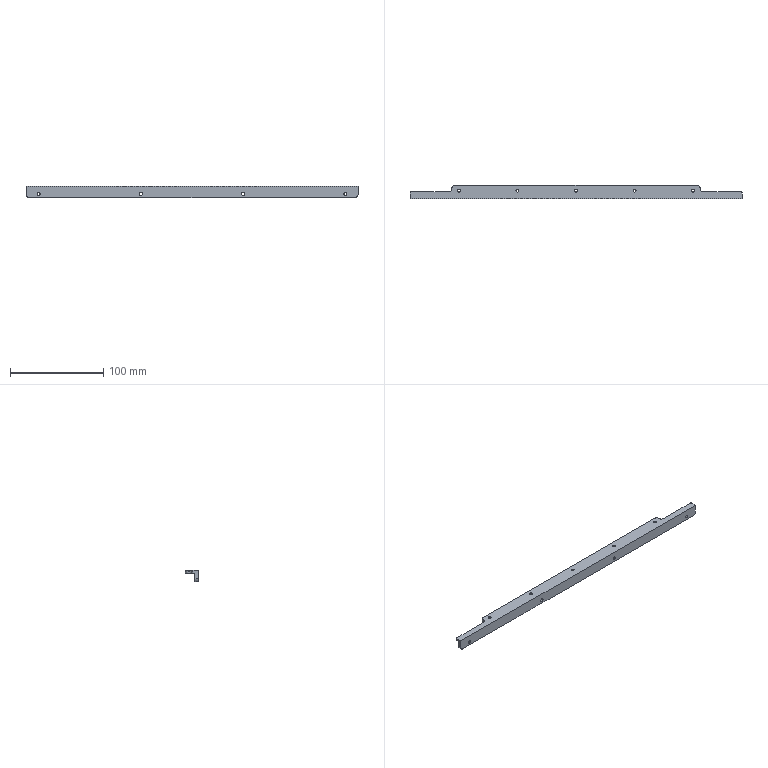NC program | NX | posted with a generic post | part box 356.96 x 14 x 12 mm
Lines 2604 to 3585 of 3585:
(PLANAR_MILL_1 , TOOL : D6精光)
N5200 T02 M6
N5202 G54
N5204 G17 G0 G90 X-181.515 Y-11.197 B0. C0. S4500 M3
N5206 G43 Z30. H2
N5208 Z-10.2
N5210 G94 G1 Z-12.2 F800.
N5212 G41 X-181.48 Y-11.
N5214 Y-6.998
N5216 Y-1.
N5218 G2 X-177.48 Y3. R4.
N5220 G1 X-136.5
N5222 Y4.
N5224 G2 X-130.5 Y10. R6.
N5226 G1 X130.5
N5228 G2 X136.5 Y4. R6.
N5230 G1 Y3.
N5232 X177.48
N5234 G2 X181.48 Y-1. R4.
N5236 G1 Y-7.
N5238 G2 X178.48 Y-10. R3.
N5240 G1 X-178.478
N5242 X-182.48
N5244 G40
N5246 X-182.677 Y-10.035
N5248 Z-10.2
N5250 G0 Z30.
N5252 X-181.515 Y-11.197
N5254 Z-10.2
N5256 G1 Z-12.2
N5258 G41 X-181.48 Y-11.
N5260 Y-6.998
N5262 Y-1.
N5264 G2 X-177.48 Y3. R4.
N5266 G1 X-136.5
N5268 Y4.
N5270 G2 X-130.5 Y10. R6.
N5272 G1 X130.5
N5274 G2 X136.5 Y4. R6.
N5276 G1 Y3.
N5278 X177.48
N5280 G2 X181.48 Y-1. R4.
N5282 G1 Y-7.
N5284 G2 X178.48 Y-10. R3.
N5286 G1 X-178.478
N5288 X-182.48
N5290 G40
N5292 X-182.677 Y-10.035
N5294 Z-10.2
N5296 G0 Z30.
(FLOOR_FACING , TOOL : D6精光)
N5298 X-137.886 Y9.315
N5300 Z-6.
N5302 G1 Z-9.
N5304 Y7.1
N5306 G3 X-136.386 Y5.6 R1.5
N5308 G1 X136.386
N5310 X177.48 Y3.1
N5312 X178.196 Y3.037
N5314 X178.89 Y2.85
N5316 X-178.89
N5318 G3 X-181.43 Y0.1 R4.1
N5320 G1 X181.43
N5322 G3 X182.93 Y1.6 R1.5
N5324 G1 Y3.551
N5326 Z-6.
N5328 G0 Z30.
(PLANAR_MILL_1_COPY , TOOL : D6精光)
N5330 X-183.677 Y0.035
N5332 Z-7.
N5334 G1 Z-9.
N5336 G41 X-183.48 Y0.
N5338 X-178.48
N5340 X178.48
N5342 X183.48
N5344 G40
N5346 X183.677 Y0.035
N5348 Z-7.
N5350 G0 Z30.
N5352 M5
(DRILLING , TOOL : D6点钻)
N5354 T03 M6
N5356 G54
N5358 G17 G0 G90 X-126. Y1.5 B0. C0. S3000 M3
N5360 G43 Z30. H3
N5362 G94 G81 G98 Z-11.5 F200. R-6.
N5364 X-63.
N5366 X0.
N5368 X63.
N5370 X126.
N5372 G80
N5374 G0 X126. Y1.5 Z30.
(PLANAR_MILL_2 , TOOL : D6点钻)
N5376 X-178.98 Y-1.5 S3500
N5378 Z0.5
N5380 G1 Z-1.5 F1000.
N5382 X-175.48
N5384 X175.48
N5386 X178.98
N5388 Z0.5
N5390 G0 Z30.
N5392 Y-8.5
N5394 Z0.5
N5396 G1 Z-1.5
N5398 X175.48
N5400 X-175.48
N5402 X-178.98
N5404 Z0.5
N5406 G0 Z30.
(PLANAR_MILL_2_COPY , TOOL : D6点钻)
N5408 X-181.48 Y2.
N5410 Z-9.
N5412 G1 Z-11.
N5414 X-177.48
N5416 X-136.5
N5418 G3 X-135.5 Y3. R1.
N5420 G1 Y4.
N5422 G2 X-130.5 Y9. R5.
N5424 G1 X130.5
N5426 G2 X135.5 Y4. R5.
N5428 G1 Y3.
N5430 G3 X136.5 Y2. R1.
N5432 G1 X177.48
N5434 X181.48
N5436 Z-9.
N5438 G0 Z30.
N5440 M5
(DRILLING_COPY , TOOL : D3.2)
N5442 T04 M6
N5444 G54
N5446 G17 G0 G90 X-126. Y1.5 B0. C0. S3000 M3
N5448 G43 Z30. H4
N5450 G94 G81 G98 Z-15. F200. R-6.
N5452 X-63.
N5454 X0.
N5456 X63.
N5458 X126.
N5460 G80
N5462 G0 X126. Y1.5 Z30.
N5464 M5
(CURVE_DRIVE , TOOL : D4R0.5)
N5466 T05 M6
N5468 G54
N5470 G17 G0 G90 X-180.431 Y-8.996 B0. C0. S4500 M3
N5472 G43 Z30. H5
N5474 Z1.526
N5476 G94 G1 Z-1.437 F1500.
N5478 X-180.433 Y-8.899 Z-2.055
N5480 X-180.439 Y-8.616 Z-2.613
N5482 X-180.448 Y-8.174 Z-3.056
N5484 X-180.46 Y-7.617 Z-3.341
N5486 X-180.473 Y-7. Z-3.44
N5488 X-180.476 Y-3.147 Z-3.441
N5490 X-180.468 Y-3.059 Z-3.44
N5492 X-180.465 Y-2.995 Z-3.474
N5494 X-180.468 Y-3.059 Z-3.44
N5496 X-180.47 Y-3.078
N5498 Y-3.106 Z-3.394
N5500 Y-3.123 Z-3.384
N5502 Y-6.878
N5504 Y-7. Z-3.408
N5506 X-180.463 Z-3.35
N5508 Y-6.845 Z-3.326
N5510 Y-3.155
N5512 Y-3.097 Z-3.331
N5514 Y-3.067 Z-3.348
N5516 Y-3.038 Z-3.387
N5518 Y-3.024 Z-3.419
N5520 Y-2.995 Z-3.456
N5522 X-180.457 Y-2.996 Z-3.346
N5524 Y-3.028 Z-3.303
N5526 Y-3.07 Z-3.279
N5528 Y-3.155 Z-3.271
N5530 Y-6.845
N5532 Y-7. Z-3.292
N5534 X-180.451 Z-3.234
N5536 Y-6.845 Z-3.215
N5538 Y-3.155
N5540 Y-3.044 Z-3.225
N5542 Y-2.997 Z-3.252
N5544 X-180.444 Y-2.998 Z-3.183
N5546 Y-3.018 Z-3.172
N5548 Y-3.155 Z-3.159
N5550 Y-6.845
N5552 Y-7. Z-3.175
N5554 X-180.437 Z-3.115
N5556 Y-6.845 Z-3.1
N5558 Y-3.155
N5560 Y-2.999 Z-3.115
N5562 X-180.43 Y-3. Z-3.055
N5564 Y-3.155 Z-3.04
N5566 Y-6.845
N5568 Y-7. Z-3.055
N5570 X-180.424 Z-2.996
N5572 Y-6.845 Z-2.981
N5574 Y-3.155
N5576 Y-3. Z-2.996
N5578 X-180.417 Z-2.936
N5580 Y-3.155 Z-2.921
N5582 Y-6.845
N5584 Y-7. Z-2.936
N5586 X-180.41 Z-2.876
N5588 Y-6.845 Z-2.862
N5590 Y-3.155
N5592 Y-3. Z-2.876
N5594 X-180.403 Y-3.001 Z-2.817
N5596 Y-3.154 Z-2.802
N5598 Y-6.842
N5600 Y-7. Z-2.817
N5602 X-180.385 Z-2.759
N5604 Y-6.845 Z-2.745
N5606 Y-3.155
N5608 Y-3.001 Z-2.759
N5610 X-180.367 Z-2.702
N5612 Y-3.155 Z-2.687
N5614 Y-6.845
N5616 Y-6.999 Z-2.702
N5618 X-180.349 Z-2.645
N5620 Y-6.845 Z-2.63
N5622 Y-3.155
N5624 Y-3.001 Z-2.645
N5626 X-180.331 Z-2.588
N5628 Y-3.155 Z-2.573
N5630 Y-6.845
N5632 Y-6.999 Z-2.588
N5634 X-180.313 Z-2.534
N5636 Y-6.845 Z-2.516
N5638 Y-3.155
N5640 Y-3.002 Z-2.534
N5642 X-180.295 Z-2.481
N5644 Y-3.067 Z-2.467
N5646 Y-3.155 Z-2.458
N5648 Y-6.845
N5650 Y-6.933 Z-2.467
N5652 Y-6.999 Z-2.481
N5654 X-180.277 Z-2.428
N5656 Y-6.897 Z-2.406
N5658 Y-6.845 Z-2.401
N5660 Y-3.155
N5662 Y-3.104 Z-2.406
N5664 Y-3.002 Z-2.428
N5666 X-180.259 Y-3.001 Z-2.375
N5668 Y-3.155 Z-2.344
N5670 Y-6.86 Z-2.345
N5672 Y-6.999 Z-2.375
N5674 X-180.238 Z-2.321
N5676 Y-6.845 Z-2.288
N5678 Y-3.155
N5680 Y-3.001 Z-2.321
N5682 X-180.216 Z-2.265
N5684 Y-3.155 Z-2.232
N5686 Y-6.845
N5688 Y-6.999 Z-2.265
N5690 X-180.193 Z-2.21
N5692 Y-6.845 Z-2.177
N5694 Y-3.155
N5696 Y-3.001 Z-2.21
N5698 X-180.17 Z-2.155
N5700 Y-3.155 Z-2.121
N5702 Y-6.845
N5704 Y-6.999 Z-2.155
N5706 X-180.147 Z-2.099
N5708 Y-6.845 Z-2.066
N5710 Y-3.155
N5712 Y-3.001 Z-2.099
N5714 X-180.124 Z-2.044
N5716 Y-3.155 Z-2.011
N5718 Y-6.845
N5720 Y-6.999 Z-2.044
N5722 X-180.102 Z-1.99
N5724 X-180.101 Y-6.84 Z-1.955
N5726 Y-3.151 Z-1.956
N5728 Y-3.001 Z-1.988
N5730 X-180.076 Z-1.932
N5732 Y-3.155 Z-1.908
N5734 Y-6.845
N5736 Y-6.999 Z-1.932
N5738 X-180.051 Z-1.878
N5740 X-180.05 Y-6.845 Z-1.857
N5742 Y-3.155
N5744 Y-3.001 Z-1.877
N5746 X-180.023 Z-1.823
N5748 Y-3.155 Z-1.804
N5750 Y-6.845
N5752 Y-7. Z-1.823
N5754 X-179.995 Z-1.77
N5756 Y-6.845 Z-1.75
N5758 Y-3.155
N5760 Y-3. Z-1.77
N5762 X-179.968 Z-1.717
N5764 Y-3.155 Z-1.697
N5766 Y-6.845
N5768 Y-7.001 Z-1.717
N5770 X-179.938 Z-1.664
N5772 Y-6.845 Z-1.647
N5774 Y-3.128 Z-1.648
N5776 Y-3. Z-1.664
N5778 X-179.904 Z-1.614
N5780 Y-3.155 Z-1.604
N5782 Y-6.94 Z-1.606
N5784 Y-7.001 Z-1.614
N5786 X-179.871 Z-1.564
N5788 Y-5. Z-1.56
N5790 Y-3. Z-1.564
N5792 X-179.834 Z-1.516
N5794 Y-5. Z-1.512
N5796 Y-7. Z-1.516
N5798 X-179.798 Z-1.469
N5800 Y-4.997 Z-1.465
N5802 Y-3. Z-1.469
N5804 X-179.761 Z-1.421
N5806 Y-5. Z-1.417
N5808 Y-7.001 Z-1.421
N5810 X-179.725 Z-1.374
N5812 Y-5. Z-1.37
N5814 Y-2.999 Z-1.374
N5816 X-179.688 Z-1.326
N5818 Y-5. Z-1.322
N5820 Y-7.001 Z-1.326
N5822 X-179.653 Z-1.28
N5824 X-179.652 Y-6.845 Z-1.274
N5826 Y-3.155
N5828 Y-2.999 Z-1.279
N5830 X-179.615 Z-1.235
N5832 Y-3.155 Z-1.227
N5834 Y-6.963 Z-1.23
N5836 Y-7.001 Z-1.235
N5838 X-179.579 Y-7.002 Z-1.191
N5840 Y-6.845 Z-1.179
N5842 Y-3.075 Z-1.181
N5844 Y-2.999 Z-1.191
N5846 X-179.542 Y-2.998 Z-1.146
N5848 Y-3.155 Z-1.132
N5850 Y-6.888 Z-1.133
N5852 Y-7.002 Z-1.146
N5854 X-179.506 Z-1.102
N5856 Y-6.851 Z-1.084
N5858 Y-3.149
N5860 Y-2.998 Z-1.102
N5862 X-179.462 Z-1.06
N5864 Y-3.155 Z-1.045
N5866 Y-6.845
N5868 Y-7.002 Z-1.06
N5870 X-179.418 Y-7.001 Z-1.02
N5872 Y-6.845 Z-1.008
N5874 Y-3.155
N5876 Y-2.999 Z-1.02
N5878 X-179.372 Y-3. Z-0.981
N5880 Y-3.155 Z-0.969
N5882 Y-6.845
N5884 Y-7.001 Z-0.981
N5886 X-179.326 Y-7. Z-0.942
N5888 Y-6.845 Z-0.931
N5890 Y-3.155
N5892 Y-3. Z-0.942
N5894 X-179.281 Y-3.001 Z-0.903
N5896 Y-3.155 Z-0.892
N5898 Y-6.845
N5900 Y-6.999 Z-0.904
N5902 X-179.235 Y-7. Z-0.865
N5904 Y-6.845 Z-0.853
N5906 Y-3.155
N5908 Y-3.001 Z-0.865
N5910 X-179.188 Z-0.827
N5912 Y-3.155 Z-0.815
N5914 Y-6.845
N5916 Y-7. Z-0.827
N5918 X-179.141 Z-0.79
N5920 Y-6.845 Z-0.779
N5922 Y-3.155
N5924 Y-3.001 Z-0.79
N5926 X-179.093 Z-0.754
N5928 Y-3.155 Z-0.742
N5930 Y-6.845
N5932 Y-7. Z-0.754
N5934 X-179.046 Z-0.717
N5936 Y-6.845 Z-0.706
N5938 Y-3.155
N5940 Y-3.001 Z-0.717
N5942 X-178.998 Z-0.681
N5944 Y-3.155 Z-0.669
N5946 Y-6.845
N5948 Y-7. Z-0.681
N5950 X-178.95 Z-0.644
N5952 Y-6.845 Z-0.633
N5954 Y-3.155
N5956 Y-3.001 Z-0.644
N5958 X-178.903 Z-0.608
N5960 Y-3.153 Z-0.596
N5962 Y-6.845
N5964 Y-7. Z-0.608
N5966 X-178.853 Z-0.574
N5968 Y-6.845 Z-0.565
N5970 Y-3.155
N5972 Y-3.001 Z-0.574
N5974 X-178.803 Z-0.541
N5976 Y-3.155 Z-0.534
N5978 Y-6.845
N5980 Y-7. Z-0.541
N5982 X-178.751 Z-0.51
N5984 Y-6.845 Z-0.503
N5986 Y-3.155
N5988 Y-3.001 Z-0.51
N5990 X-178.7 Y-3. Z-0.479
N5992 Y-3.155 Z-0.472
N5994 Y-6.845
N5996 Y-7. Z-0.479
N5998 X-178.649 Z-0.448
N6000 Y-6.845 Z-0.441
N6002 Y-3.155
N6004 Y-3. Z-0.447
N6006 X-178.598 Z-0.416
N6008 Y-3.154 Z-0.41
N6010 Y-6.843
N6012 Y-7. Z-0.416
N6014 X-178.542 Z-0.393
N6016 Y-6.845 Z-0.387
N6018 Y-3.155
N6020 Y-3. Z-0.393
N6022 X-178.487 Z-0.37
N6024 Y-3.155 Z-0.364
N6026 Y-6.845
N6028 Y-7. Z-0.37
N6030 X-178.431 Z-0.347
N6032 Y-6.845 Z-0.341
N6034 Y-3.155
N6036 Y-3. Z-0.347
N6038 X-178.376 Z-0.324
N6040 Y-3.155 Z-0.318
N6042 Y-6.845
N6044 Y-7. Z-0.324
N6046 X-178.321 Z-0.301
N6048 Y-6.845 Z-0.295
N6050 Y-3.155
N6052 Y-3. Z-0.301
N6054 X-178.265 Z-0.278
N6056 Y-3.155 Z-0.272
N6058 Y-6.845
N6060 Y-7. Z-0.278
N6062 X-178.21 Z-0.255
N6064 Y-6.845 Z-0.249
N6066 Y-3.155
N6068 Y-3. Z-0.255
N6070 X-178.154 Z-0.232
N6072 Y-3.155 Z-0.226
N6074 Y-6.845
N6076 Y-7. Z-0.232
N6078 X-178.099 Z-0.21
N6080 Y-6.845 Z-0.203
N6082 Y-3.155
N6084 Y-3. Z-0.21
N6086 X-178.043 Z-0.187
N6088 Y-3.155 Z-0.18
N6090 Y-6.845
N6092 Y-7.001 Z-0.187
N6094 X-177.988 Z-0.164
N6096 Y-6.845 Z-0.158
N6098 Y-3.151
N6100 Y-3. Z-0.164
N6102 X-177.93 Z-0.147
N6104 Y-6.845 Z-0.143
N6106 Y-7.001 Z-0.147
N6108 X-177.873 Y-7. Z-0.131
N6110 Y-3.
N6112 X-177.815 Z-0.115
N6114 Y-7.
N6116 X-177.757 Z-0.1
N6118 Y-3.
N6120 X-177.699 Z-0.085
N6122 Y-7.
N6124 X-177.64 Z-0.073
N6126 Y-3.
N6128 X-177.581 Z-0.062
N6130 Y-7.
N6132 X-177.522 Z-0.051
N6134 Y-3.
N6136 X-177.463 Z-0.04
N6138 Y-7.
N6140 X-177.404 Z-0.03
N6142 Y-3.
N6144 X-177.344 Z-0.025
N6146 Y-7.
N6148 X-177.284 Z-0.022
N6150 Y-3.
N6152 X-177.224 Z-0.019
N6154 Y-7.
N6156 X-177.164 Z-0.016
N6158 Y-3.
N6160 X-177.104 Z-0.014
N6162 Y-7.
N6164 X-177.044 Z-0.011
N6166 Y-3.
N6168 X-176.984 Z-0.008
N6170 Y-7.
N6172 X-176.924 Z-0.006
N6174 Y-3.
N6176 X-176.864 Z-0.003
N6178 Y-7.
N6180 X-176.804 Z-0.001
N6182 Y-3.
N6184 X-176.744 Z0.
N6186 Y-7.
N6188 X-176.684
N6190 Y-3.
N6192 X-176.624
N6194 Y-7.
N6196 X-176.564
N6198 Y-3.
N6200 X-176.504
N6202 Y-7.
N6204 X-176.444
N6206 Y-3.
N6208 X-176.384
N6210 Y-7.
N6212 X-176.324
N6214 Y-3.
N6216 X-176.264
N6218 Y-7.
N6220 X-176.204
N6222 Y-3.
N6224 X-176.144
N6226 Y-7.
N6228 X-176.084
N6230 Y-3.
N6232 X-176.024
N6234 Y-7.
N6236 X-175.964
N6238 Y-3.
N6240 X-175.904
N6242 Y-7.
N6244 X-175.844
N6246 Y-3.
N6248 X-175.784
N6250 Y-7.
N6252 X-175.724
N6254 Y-3.
N6256 X-175.664
N6258 Y-7.
N6260 X-175.604
N6262 Y-3.
N6264 X-175.544
N6266 Y-7.
N6268 Y-7.618 Z0.098
N6270 Y-8.176 Z0.382
N6272 Y-8.618 Z0.824
N6274 Y-8.902 Z1.382
N6276 Y-9. Z2.
N6278 Z2.931
N6280 G0 Z30.
N6282 X175.57
N6284 Z2.93
N6286 G1 Z2.
N6288 Y-8.902 Z1.382
N6290 Y-8.618 Z0.824
N6292 Y-8.176 Z0.382
N6294 Y-7.618 Z0.098
N6296 Y-7. Z0.
N6298 Y-3.
N6300 X175.63
N6302 Y-7.
N6304 X175.69
N6306 Y-3.
N6308 X175.75
N6310 Y-7.
N6312 X175.81
N6314 Y-3.
N6316 X175.87
N6318 Y-7.
N6320 X175.93
N6322 Y-3.
N6324 X175.99
N6326 Y-7.
N6328 X176.05
N6330 Y-3.
N6332 X176.11
N6334 Y-7.
N6336 X176.17
N6338 Y-3.
N6340 X176.23
N6342 Y-7.
N6344 X176.29
N6346 Y-3.
N6348 X176.35
N6350 Y-7.
N6352 X176.41
N6354 Y-3.
N6356 X176.47
N6358 Y-7.
N6360 X176.53
N6362 Y-3.
N6364 X176.59
N6366 Y-7.
N6368 X176.65
N6370 Y-3.
N6372 X176.71
N6374 Y-7.
N6376 X176.77
N6378 Y-3.
N6380 X176.83 Z-0.002
N6382 Y-7.
N6384 X176.89 Z-0.004
N6386 Y-3.
N6388 X176.95 Z-0.007
N6390 Y-7.
N6392 X177.01 Z-0.009
N6394 Y-3.
N6396 X177.07 Z-0.012
N6398 Y-7.
N6400 X177.13 Z-0.015
N6402 Y-3.
N6404 X177.19 Z-0.017
N6406 Y-7.
N6408 X177.249 Z-0.02
N6410 Y-3.
N6412 X177.309 Z-0.023
N6414 Y-7.
N6416 X177.369 Z-0.027
N6418 Y-3.
N6420 X177.429 Z-0.034
N6422 Y-7.
N6424 X177.488 Z-0.045
N6426 Y-3.
N6428 X177.547 Z-0.056
N6430 Y-7.
N6432 X177.606 Z-0.066
N6434 Y-3.
N6436 X177.665 Z-0.078
N6438 Y-7.
N6440 X177.723 Z-0.091
N6442 Y-3.
N6444 X177.781 Z-0.107
N6446 Y-7.
N6448 X177.839 Z-0.122
N6450 Y-3.
N6452 X177.897 Z-0.137
N6454 Y-7.001
N6456 X177.955 Z-0.154
N6458 Y-6.845 Z-0.149
N6460 Y-3.074 Z-0.151
N6462 Y-3. Z-0.154
N6464 X178.012 Z-0.173
N6466 Y-3.155 Z-0.167
N6468 Y-6.845
N6470 Y-7.001 Z-0.173
N6472 X178.067 Z-0.196
N6474 Y-6.845 Z-0.19
N6476 Y-3.155
N6478 Y-3. Z-0.196
N6480 X178.123 Z-0.219
N6482 Y-3.155 Z-0.213
N6484 Y-6.845
N6486 Y-7. Z-0.219
N6488 X178.178 Z-0.242
N6490 Y-6.845 Z-0.236
N6492 Y-3.155
N6494 Y-3. Z-0.242
N6496 X178.233 Z-0.265
N6498 Y-3.155 Z-0.259
N6500 Y-6.845
N6502 Y-7. Z-0.265
N6504 X178.289 Z-0.288
N6506 Y-6.845 Z-0.282
N6508 Y-3.155
N6510 Y-3. Z-0.288
N6512 X178.344 Z-0.311
N6514 Y-3.155 Z-0.305
N6516 Y-6.845
N6518 Y-7. Z-0.311
N6520 X178.4 Z-0.334
N6522 Y-6.845 Z-0.327
N6524 Y-3.155
N6526 Y-3. Z-0.334
N6528 X178.455 Z-0.357
N6530 Y-3.155 Z-0.35
N6532 Y-6.845
N6534 Y-7. Z-0.357
N6536 X178.511 Z-0.38
N6538 Y-6.845 Z-0.373
N6540 Y-3.155
N6542 Y-3. Z-0.38
N6544 X178.566 Z-0.403
N6546 Y-3.155 Z-0.396
N6548 Y-6.845
N6550 Y-7. Z-0.403
N6552 X178.62 Z-0.43
N6554 Y-6.845 Z-0.423
N6556 Y-3.155
N6558 Y-3. Z-0.43
N6560 X178.671 Z-0.461
N6562 Y-3.155 Z-0.454
N6564 Y-6.845
N6566 Y-7. Z-0.461
N6568 X178.722 Z-0.492
N6570 Y-6.845 Z-0.485
N6572 Y-3.155
N6574 Y-3.001 Z-0.492
N6576 X178.773 Z-0.523
N6578 Y-3.155 Z-0.517
N6580 Y-6.845
N6582 Y-7. Z-0.523
N6584 X178.825 Z-0.555
N6586 Y-6.845 Z-0.548
N6588 Y-3.155
N6590 Y-3.001 Z-0.555
N6592 X178.874 Z-0.588
N6594 Y-3.155 Z-0.578
N6596 Y-6.892 Z-0.58
N6598 Y-7. Z-0.588
N6600 X178.923 Z-0.623
N6602 Y-6.845 Z-0.612
N6604 Y-3.155
N6606 Y-3.001 Z-0.623
N6608 X178.971 Z-0.66
N6610 Y-3.155 Z-0.648
N6612 Y-6.845
N6614 Y-7. Z-0.66
N6616 X179.018 Z-0.696
N6618 Y-6.845 Z-0.685
N6620 Y-3.155
N6622 Y-3.001 Z-0.696
N6624 X179.066 Z-0.733
N6626 Y-3.155 Z-0.721
N6628 Y-6.845
N6630 Y-7. Z-0.733
N6632 X179.113 Z-0.769
N6634 Y-6.845 Z-0.758
N6636 Y-3.155
N6638 Y-3.001 Z-0.769
N6640 X179.161 Z-0.806
N6642 Y-3.155 Z-0.794
N6644 Y-6.845
N6646 Y-7. Z-0.806
N6648 X179.208 Z-0.843
N6650 Y-6.845 Z-0.831
N6652 Y-3.155
N6654 Y-3.001 Z-0.843
N6656 X179.254 Z-0.881
N6658 Y-3.155 Z-0.87
N6660 Y-6.845
N6662 Y-7. Z-0.881
N6664 X179.3 Z-0.92
N6666 Y-6.845 Z-0.909
N6668 Y-3.155
N6670 Y-3.001 Z-0.92
N6672 X179.346 Y-3. Z-0.959
N6674 Y-3.155 Z-0.947
N6676 Y-6.845
N6678 Y-7. Z-0.959
N6680 X179.392 Y-7.001 Z-0.997
N6682 Y-6.845 Z-0.986
N6684 Y-3.155
N6686 Y-2.999 Z-0.997
N6688 X179.437 Z-1.037
N6690 Y-3.155 Z-1.024
N6692 Y-6.845
N6694 Y-7.002 Z-1.037
N6696 X179.481 Z-1.078
N6698 Y-6.845 Z-1.061
N6700 Y-3.117 Z-1.064
N6702 Y-2.998 Z-1.078
N6704 X179.521 Z-1.122
N6706 Y-3.155 Z-1.105
N6708 Y-6.867 Z-1.106
N6710 Y-7.002 Z-1.122
N6712 X179.558 Z-1.166
N6714 Y-6.845 Z-1.153
N6716 Y-3.095 Z-1.154
N6718 Y-2.998 Z-1.166
N6720 X179.595 Y-2.999 Z-1.21
N6722 Y-3.155 Z-1.2
N6724 Y-6.942 Z-1.203
N6726 Y-7.002 Z-1.21
N6728 X179.631 Y-7.001 Z-1.254
N6730 Y-6.845 Z-1.248
N6732 Y-3.021 Z-1.251
N6734 Y-2.999 Z-1.254
N6736 X179.668 Z-1.299
N6738 Y-5. Z-1.295
N6740 Y-7.001 Z-1.299
N6742 X179.704 Z-1.347
N6744 Y-5. Z-1.343
N6746 Y-2.999 Z-1.347
N6748 X179.741 Y-3. Z-1.395
N6750 Y-5. Z-1.391
N6752 Y-7.001 Z-1.395
N6754 X179.777 Y-7. Z-1.442
N6756 Y-5. Z-1.438
N6758 Y-3. Z-1.442
N6760 X179.814 Z-1.49
N6762 Y-5. Z-1.486
N6764 Y-7. Z-1.49
N6766 X179.85 Y-7.001 Z-1.537
N6768 Y-5. Z-1.533
N6770 Y-3. Z-1.537
N6772 X179.886 Z-1.586
N6774 Y-3.155 Z-1.58
N6776 Y-6.978 Z-1.583
N6778 Y-7.001 Z-1.586
N6780 X179.919 Z-1.636
N6782 Y-6.911 Z-1.624
N6784 Y-3.089
N6786 Y-3. Z-1.636
N6788 X179.951 Z-1.684
N6790 X179.952 Y-3.154 Z-1.666
N6792 Y-6.845
N6794 Y-7.001 Z-1.686
N6796 X179.979 Y-7. Z-1.739
N6798 Y-6.845 Z-1.72
N6800 Y-3.155
N6802 Y-3. Z-1.739
N6804 X180.007 Z-1.793
N6806 Y-3.155 Z-1.773
N6808 Y-6.845
N6810 Y-7. Z-1.793
N6812 X180.034 Z-1.846
N6814 Y-6.845 Z-1.826
N6816 Y-3.155
N6818 Y-3.001 Z-1.846
N6820 X180.062 Z-1.899
N6822 Y-3.155 Z-1.88
N6824 Y-6.845
N6826 Y-6.999 Z-1.899
N6828 X180.086 Z-1.954
N6830 Y-6.845 Z-1.927
N6832 Y-3.155
N6834 Y-3.001 Z-1.954
N6836 X180.109 Z-2.009
N6838 Y-3.155 Z-1.976
N6840 Y-6.845
N6842 Y-6.999 Z-2.009
N6844 X180.132 Z-2.065
N6846 Y-6.845 Z-2.032
N6848 Y-3.155
N6850 Y-3.001 Z-2.065
N6852 X180.155 Z-2.12
N6854 Y-3.155 Z-2.087
N6856 Y-6.845
N6858 Y-6.999 Z-2.12
N6860 X180.178 Z-2.176
N6862 Y-6.845 Z-2.142
N6864 Y-3.155
N6866 Y-3.001 Z-2.175
N6868 X180.201 Z-2.231
N6870 Y-3.155 Z-2.198
N6872 Y-6.845
N6874 Y-6.999 Z-2.231
N6876 X180.224 Z-2.286
N6878 Y-6.845 Z-2.253
N6880 Y-3.155
N6882 Y-3.001 Z-2.286
N6884 X180.247 Z-2.342
N6886 Y-3.155 Z-2.309
N6888 Y-6.845
N6890 Y-6.999 Z-2.342
N6892 X180.266 Z-2.395
N6894 Y-6.845 Z-2.366
N6896 Y-3.126 Z-2.368
N6898 Y-3.001 Z-2.395
N6900 X180.284 Z-2.448
N6902 Y-3.089 Z-2.429
N6904 Y-3.155 Z-2.423
N6906 Y-6.845
N6908 Y-6.911 Z-2.429
N6910 Y-6.999 Z-2.448
N6912 X180.302 Z-2.499
N6914 Y-6.845 Z-2.48
N6916 Y-3.155
N6918 Y-3.052 Z-2.49
N6920 Y-3.002 Z-2.501
N6922 X180.32 Y-3.001 Z-2.554
N6924 Y-3.155 Z-2.537
N6926 Y-6.845
N6928 Y-6.999 Z-2.554
N6930 X180.338 Z-2.609
N6932 Y-6.845 Z-2.595
N6934 Y-3.155
N6936 Y-3.001 Z-2.609
N6938 X180.356 Z-2.666
N6940 Y-3.155 Z-2.652
N6942 Y-6.845
N6944 Y-6.999 Z-2.666
N6946 X180.374 Y-7. Z-2.724
N6948 Y-6.845 Z-2.709
N6950 Y-3.155
N6952 Y-3.001 Z-2.724
N6954 X180.392 Y-3. Z-2.781
N6956 Y-3.155 Z-2.766
N6958 Y-6.845
N6960 Y-7. Z-2.781
N6962 X180.405 Z-2.839
N6964 Y-6.845 Z-2.825
N6966 Y-3.155
N6968 Y-3. Z-2.839
N6970 X180.412 Z-2.899
N6972 Y-3.155 Z-2.884
N6974 Y-6.845
N6976 Y-7. Z-2.899
N6978 X180.419 Z-2.959
N6980 Y-6.845 Z-2.944
N6982 Y-3.155
N6984 Y-3. Z-2.959
N6986 X180.426 Z-3.018
N6988 Y-3.155 Z-3.003
N6990 Y-6.845
N6992 Y-7. Z-3.018
N6994 X180.433 Z-3.078
N6996 Y-6.845 Z-3.063
N6998 Y-3.155
N7000 Y-3. Z-3.078
N7002 X180.44 Z-3.135
N7004 Y-3.155 Z-3.122
N7006 Y-6.845
N7008 Y-7. Z-3.137
N7010 X180.446 Z-3.188
N7012 Y-6.845 Z-3.171
N7014 Y-3.155
N7016 Y-3.024 Z-3.183
N7018 Y-3. Z-3.197
N7020 X180.451 Z-3.257
N7022 Y-3.047 Z-3.23
N7024 Y-3.155 Z-3.219
N7026 Y-6.845
N7028 Y-7. Z-3.239
N7030 X180.456 Z-3.278
N7032 Y-6.845 Z-3.257
N7034 Y-3.155
N7036 Y-3.065 Z-3.265
N7038 Y-3.02 Z-3.292
N7040 Y-3. Z-3.317
N7042 X180.459 Y-3.001 Z-3.377
N7044 Y-3.043 Z-3.318
N7046 Y-3.08 Z-3.296
N7048 Y-3.155 Z-3.289
N7050 Y-6.845
N7052 Y-7. Z-3.312
N7054 X180.463 Z-3.342
N7056 Y-6.845 Z-3.318
N7058 Y-3.155
N7060 Y-3.094 Z-3.324
N7062 Y-3.063 Z-3.342
N7064 Y-3.033 Z-3.382
N7066 Y-3.001 Z-3.437
N7068 X180.466 Z-3.481
N7070 X180.469 Y-3.039 Z-3.482
N7072 Y-3.067 Z-3.445
N7074 Y-3.084 Z-3.41
N7076 Y-3.102 Z-3.386
N7078 Y-3.12 Z-3.376
N7080 Y-6.88
N7082 Y-7. Z-3.399
N7084 X180.475 Z-3.456
N7086 X180.476 Y-6.845 Z-3.432
N7088 Y-3.143 Z-3.434
N7090 X180.475 Y-3.113 Z-3.484
N7092 X180.48 Y-3.334 Z-3.492
N7094 Y-6.845 Z-3.493
N7096 X180.479 Y-6.892 Z-3.5
N7098 X180.472 Y-7.517 Z-3.498
N7100 X180.465 Y-8.112 Z-3.303
N7102 X180.459 Y-8.617 Z-2.933
N7104 X180.454 Y-8.983 Z-2.426
N7106 X180.452 Y-9.174 Z-1.83
N7108 Z1.421
N7110 G0 Z30.
N7112 M5
N7114 M2